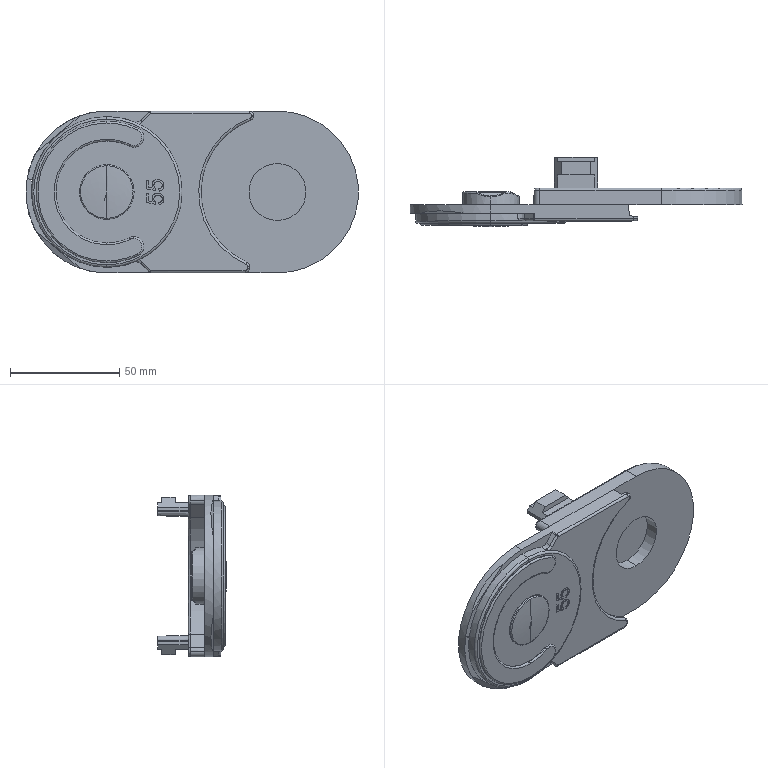Part | SolidWorks | features BaseBody 1 | 1 solid | 281 faces | box 152 x 31.5 x 74 mm | volume 87021 mm3 | plane 112 | spline 53 | cylinder 47 | cone 42 | torus 19 | sphere 8 | commonest cylinder face diameters 2 x12 6 x6 4 x4 5 x4 9 x3 46.703 x3